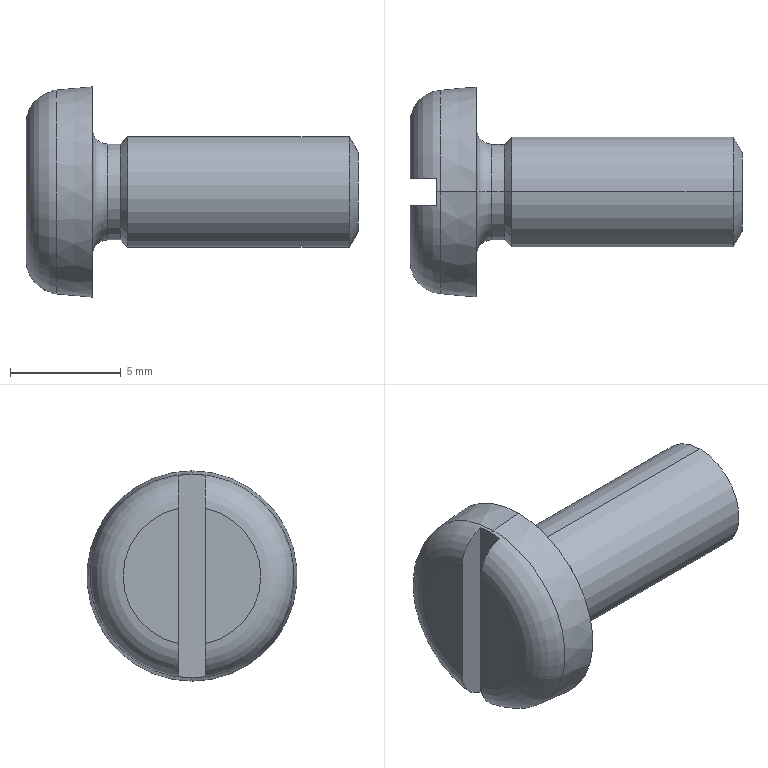Part | SolidWorks | features Cut 1, LPattern 1, RevCut 1, Revolution 1 | 1 solid | 21 faces | box 15 x 9.5 x 9.5 mm | volume 406.666 mm3 | plane 7 | cone 6 | cylinder 4 | torus 4 | commonest cylinder face diameters 4.33 x2 5 x2
STEP:
#1=CARTESIAN_POINT('',(15.,0.,-1.807));
#2=VERTEX_POINT('',#1);
#3=CARTESIAN_POINT('',(15.,0.,1.807));
#4=VERTEX_POINT('',#3);
#5=CARTESIAN_POINT('',(15.,0.,0.));
#6=DIRECTION('',(1.,0.,0.));
#7=DIRECTION('',(0.,0.,-1.));
#8=AXIS2_PLACEMENT_3D('',#5,#6,#7);
#9=CIRCLE('',#8,1.807);
#10=EDGE_CURVE('',#2,#4,#9,.T.);
#11=ORIENTED_EDGE('',*,*,#10,.F.);
#12=CARTESIAN_POINT('',(14.596,0.,-2.5));
#13=VERTEX_POINT('',#12);
#14=CARTESIAN_POINT('',(14.596,0.,-2.5));
#15=DIRECTION('',(-0.5041,0.,-0.8637));
#16=VECTOR('',#15,1000.);
#17=LINE('',#14,#16);
#18=EDGE_CURVE('',#2,#13,#17,.T.);
#19=ORIENTED_EDGE('',*,*,#18,.T.);
#20=CARTESIAN_POINT('',(14.596,0.,2.5));
#21=VERTEX_POINT('',#20);
#22=CARTESIAN_POINT('',(14.596,0.,0.));
#23=DIRECTION('',(1.,0.,0.));
#24=DIRECTION('',(0.,0.,-1.));
#25=AXIS2_PLACEMENT_3D('',#22,#23,#24);
#26=CIRCLE('',#25,2.5);
#27=EDGE_CURVE('',#13,#21,#26,.T.);
#28=ORIENTED_EDGE('',*,*,#27,.T.);
#29=CARTESIAN_POINT('',(14.596,0.,2.5));
#30=DIRECTION('',(-0.5041,0.,0.8637));
#31=VECTOR('',#30,1000.);
#32=LINE('',#29,#31);
#33=EDGE_CURVE('',#4,#21,#32,.T.);
#34=ORIENTED_EDGE('',*,*,#33,.F.);
#35=EDGE_LOOP('',(#11,#19,#28,#34));
#36=FACE_OUTER_BOUND('',#35,.T.);
#37=CARTESIAN_POINT('',(14.596,0.,0.));
#38=DIRECTION('',(-1.,0.,0.));
#39=DIRECTION('',(0.,0.,1.));
#40=AXIS2_PLACEMENT_3D('',#37,#38,#39);
#41=CONICAL_SURFACE('',#40,2.5,1.043);
#42=ADVANCED_FACE('',(#36),#41,.T.);
#43=ORIENTED_EDGE('',*,*,#27,.F.);
#44=CARTESIAN_POINT('',(4.6,0.,-2.5));
#45=VERTEX_POINT('',#44);
#46=CARTESIAN_POINT('',(-2.477,0.,-2.5));
#47=DIRECTION('',(-1.,0.,0.));
#48=VECTOR('',#47,1000.);
#49=LINE('',#46,#48);
#50=EDGE_CURVE('',#13,#45,#49,.T.);
#51=ORIENTED_EDGE('',*,*,#50,.T.);
#52=CARTESIAN_POINT('',(4.6,0.,2.5));
#53=VERTEX_POINT('',#52);
#54=CARTESIAN_POINT('',(4.6,0.,0.));
#55=DIRECTION('',(-1.,0.,0.));
#56=DIRECTION('',(0.,0.,1.));
#57=AXIS2_PLACEMENT_3D('',#54,#55,#56);
#58=CIRCLE('',#57,2.5);
#59=EDGE_CURVE('',#53,#45,#58,.T.);
#60=ORIENTED_EDGE('',*,*,#59,.F.);
#61=CARTESIAN_POINT('',(-2.477,0.,2.5));
#62=DIRECTION('',(-1.,0.,0.));
#63=VECTOR('',#62,1000.);
#64=LINE('',#61,#63);
#65=EDGE_CURVE('',#21,#53,#64,.T.);
#66=ORIENTED_EDGE('',*,*,#65,.F.);
#67=EDGE_LOOP('',(#43,#51,#60,#66));
#68=FACE_OUTER_BOUND('',#67,.T.);
#69=CARTESIAN_POINT('',(-2.477,0.,0.));
#70=DIRECTION('',(-1.,0.,0.));
#71=DIRECTION('',(0.,0.,1.));
#72=AXIS2_PLACEMENT_3D('',#69,#70,#71);
#73=CYLINDRICAL_SURFACE('',#72,2.5);
#74=ADVANCED_FACE('',(#68),#73,.T.);
#75=CARTESIAN_POINT('',(4.265,0.,2.165));
#76=VERTEX_POINT('',#75);
#77=CARTESIAN_POINT('',(4.265,0.,-2.165));
#78=VERTEX_POINT('',#77);
#79=CARTESIAN_POINT('',(4.265,0.,0.));
#80=DIRECTION('',(-1.,0.,0.));
#81=DIRECTION('',(0.,0.,1.));
#82=AXIS2_PLACEMENT_3D('',#79,#80,#81);
#83=CIRCLE('',#82,2.165);
#84=EDGE_CURVE('',#76,#78,#83,.T.);
#85=ORIENTED_EDGE('',*,*,#84,.F.);
#86=CARTESIAN_POINT('',(4.6,0.,2.5));
#87=DIRECTION('',(0.7071,0.,0.7071));
#88=VECTOR('',#87,1000.);
#89=LINE('',#86,#88);
#90=EDGE_CURVE('',#76,#53,#89,.T.);
#91=ORIENTED_EDGE('',*,*,#90,.T.);
#92=ORIENTED_EDGE('',*,*,#59,.T.);
#93=CARTESIAN_POINT('',(4.6,0.,-2.5));
#94=DIRECTION('',(0.7071,0.,-0.7071));
#95=VECTOR('',#94,1000.);
#96=LINE('',#93,#95);
#97=EDGE_CURVE('',#78,#45,#96,.T.);
#98=ORIENTED_EDGE('',*,*,#97,.F.);
#99=EDGE_LOOP('',(#85,#91,#92,#98));
#100=FACE_OUTER_BOUND('',#99,.T.);
#101=CARTESIAN_POINT('',(4.6,0.,0.));
#102=DIRECTION('',(1.,0.,0.));
#103=DIRECTION('',(0.,0.,-1.));
#104=AXIS2_PLACEMENT_3D('',#101,#102,#103);
#105=CONICAL_SURFACE('',#104,2.5,0.7854);
#106=ADVANCED_FACE('',(#100),#105,.T.);
#107=ORIENTED_EDGE('',*,*,#84,.T.);
#108=CARTESIAN_POINT('',(3.685,0.,-2.165));
#109=VERTEX_POINT('',#108);
#110=CARTESIAN_POINT('',(-2.477,0.,-2.165));
#111=DIRECTION('',(-1.,0.,0.));
#112=VECTOR('',#111,1000.);
#113=LINE('',#110,#112);
#114=EDGE_CURVE('',#78,#109,#113,.T.);
#115=ORIENTED_EDGE('',*,*,#114,.T.);
#116=CARTESIAN_POINT('',(3.685,0.,2.165));
#117=VERTEX_POINT('',#116);
#118=CARTESIAN_POINT('',(3.685,0.,0.));
#119=DIRECTION('',(-1.,0.,0.));
#120=DIRECTION('',(0.,0.,1.));
#121=AXIS2_PLACEMENT_3D('',#118,#119,#120);
#122=CIRCLE('',#121,2.165);
#123=EDGE_CURVE('',#117,#109,#122,.T.);
#124=ORIENTED_EDGE('',*,*,#123,.F.);
#125=CARTESIAN_POINT('',(-2.477,0.,2.165));
#126=DIRECTION('',(-1.,0.,0.));
#127=VECTOR('',#126,1000.);
#128=LINE('',#125,#127);
#129=EDGE_CURVE('',#76,#117,#128,.T.);
#130=ORIENTED_EDGE('',*,*,#129,.F.);
#131=EDGE_LOOP('',(#107,#115,#124,#130));
#132=FACE_OUTER_BOUND('',#131,.T.);
#133=CARTESIAN_POINT('',(-2.477,0.,0.));
#134=DIRECTION('',(-1.,0.,0.));
#135=DIRECTION('',(0.,0.,1.));
#136=AXIS2_PLACEMENT_3D('',#133,#134,#135);
#137=CYLINDRICAL_SURFACE('',#136,2.165);
#138=ADVANCED_FACE('',(#132),#137,.T.);
#139=CARTESIAN_POINT('',(3.,0.,-2.85));
#140=VERTEX_POINT('',#139);
#141=CARTESIAN_POINT('',(3.,0.,2.85));
#142=VERTEX_POINT('',#141);
#143=CARTESIAN_POINT('',(3.,0.,0.));
#144=DIRECTION('',(-1.,0.,0.));
#145=DIRECTION('',(0.,0.,1.));
#146=AXIS2_PLACEMENT_3D('',#143,#144,#145);
#147=CIRCLE('',#146,2.85);
#148=EDGE_CURVE('',#140,#142,#147,.T.);
#149=ORIENTED_EDGE('',*,*,#148,.F.);
#150=CARTESIAN_POINT('',(3.685,0.,-2.85));
#151=DIRECTION('',(0.,1.,0.));
#152=DIRECTION('',(0.,0.,1.));
#153=AXIS2_PLACEMENT_3D('',#150,#151,#152);
#154=CIRCLE('',#153,0.685);
#155=EDGE_CURVE('',#140,#109,#154,.T.);
#156=ORIENTED_EDGE('',*,*,#155,.T.);
#157=CARTESIAN_POINT('',(3.685,0.,0.));
#158=DIRECTION('',(-1.,0.,0.));
#159=DIRECTION('',(0.,0.,1.));
#160=AXIS2_PLACEMENT_3D('',#157,#158,#159);
#161=CIRCLE('',#160,2.165);
#162=EDGE_CURVE('',#109,#117,#161,.T.);
#163=ORIENTED_EDGE('',*,*,#162,.T.);
#164=CARTESIAN_POINT('',(3.685,0.,2.85));
#165=DIRECTION('',(0.,-1.,0.));
#166=DIRECTION('',(1.,0.,0.));
#167=AXIS2_PLACEMENT_3D('',#164,#165,#166);
#168=CIRCLE('',#167,0.685);
#169=EDGE_CURVE('',#142,#117,#168,.T.);
#170=ORIENTED_EDGE('',*,*,#169,.F.);
#171=EDGE_LOOP('',(#149,#156,#163,#170));
#172=FACE_OUTER_BOUND('',#171,.T.);
#173=CARTESIAN_POINT('',(3.685,0.,0.));
#174=DIRECTION('',(-1.,0.,0.));
#175=DIRECTION('',(0.,0.,1.));
#176=AXIS2_PLACEMENT_3D('',#173,#174,#175);
#177=TOROIDAL_SURFACE('',#176,2.85,0.685);
#178=ADVANCED_FACE('',(#172),#177,.F.);
#179=CARTESIAN_POINT('',(1.369,0.,4.607));
#180=VERTEX_POINT('',#179);
#181=CARTESIAN_POINT('',(1.369,0.,-4.607));
#182=VERTEX_POINT('',#181);
#183=CARTESIAN_POINT('',(1.369,0.,0.));
#184=DIRECTION('',(-1.,0.,0.));
#185=DIRECTION('',(0.,0.,1.));
#186=AXIS2_PLACEMENT_3D('',#183,#184,#185);
#187=CIRCLE('',#186,4.607);
#188=EDGE_CURVE('',#180,#182,#187,.T.);
#189=ORIENTED_EDGE('',*,*,#188,.F.);
#190=CARTESIAN_POINT('',(3.,0.,4.75));
#191=VERTEX_POINT('',#190);
#192=CARTESIAN_POINT('',(3.,0.,4.75));
#193=DIRECTION('',(0.9962,0.,0.08716));
#194=VECTOR('',#193,1000.);
#195=LINE('',#192,#194);
#196=EDGE_CURVE('',#180,#191,#195,.T.);
#197=ORIENTED_EDGE('',*,*,#196,.T.);
#198=CARTESIAN_POINT('',(3.,0.,-4.75));
#199=VERTEX_POINT('',#198);
#200=CARTESIAN_POINT('',(3.,0.,0.));
#201=DIRECTION('',(-1.,0.,0.));
#202=DIRECTION('',(0.,0.,1.));
#203=AXIS2_PLACEMENT_3D('',#200,#201,#202);
#204=CIRCLE('',#203,4.75);
#205=EDGE_CURVE('',#191,#199,#204,.T.);
#206=ORIENTED_EDGE('',*,*,#205,.T.);
#207=CARTESIAN_POINT('',(3.,0.,-4.75));
#208=DIRECTION('',(0.9962,0.,-0.08716));
#209=VECTOR('',#208,1000.);
#210=LINE('',#207,#209);
#211=EDGE_CURVE('',#182,#199,#210,.T.);
#212=ORIENTED_EDGE('',*,*,#211,.F.);
#213=EDGE_LOOP('',(#189,#197,#206,#212));
#214=FACE_OUTER_BOUND('',#213,.T.);
#215=CARTESIAN_POINT('',(3.,0.,0.));
#216=DIRECTION('',(1.,0.,0.));
#217=DIRECTION('',(0.,0.,-1.));
#218=AXIS2_PLACEMENT_3D('',#215,#216,#217);
#219=CONICAL_SURFACE('',#218,4.75,0.08727);
#220=ADVANCED_FACE('',(#214),#219,.T.);
#221=ORIENTED_EDGE('',*,*,#188,.T.);
#222=CARTESIAN_POINT('',(1.2,0.,-4.583));
#223=VERTEX_POINT('',#222);
#224=CARTESIAN_POINT('',(1.5,0.,-3.113));
#225=DIRECTION('',(0.,1.,0.));
#226=DIRECTION('',(0.,0.,1.));
#227=AXIS2_PLACEMENT_3D('',#224,#225,#226);
#228=CIRCLE('',#227,1.5);
#229=EDGE_CURVE('',#182,#223,#228,.T.);
#230=ORIENTED_EDGE('',*,*,#229,.T.);
#231=CARTESIAN_POINT('',(1.2,0.6,-4.543));
#232=VERTEX_POINT('',#231);
#233=CARTESIAN_POINT('',(1.2,0.,0.));
#234=DIRECTION('',(1.,0.,0.));
#235=DIRECTION('',(0.,1.,0.));
#236=AXIS2_PLACEMENT_3D('',#233,#234,#235);
#237=CIRCLE('',#236,4.583);
#238=EDGE_CURVE('',#223,#232,#237,.T.);
#239=ORIENTED_EDGE('',*,*,#238,.T.);
#240=CARTESIAN_POINT('',(0.,0.6,-3.055));
#241=VERTEX_POINT('',#240);
#242=CARTESIAN_POINT('',(1.2,0.6,-4.543));
#243=CARTESIAN_POINT('',(1.03,0.6,-4.508));
#244=CARTESIAN_POINT('',(0.8696,0.6,-4.445));
#245=CARTESIAN_POINT('',(0.5733,0.6,-4.263));
#246=CARTESIAN_POINT('',(0.4414,0.6,-4.146));
#247=CARTESIAN_POINT('',(0.2269,0.6,-3.878));
#248=CARTESIAN_POINT('',(0.1419,0.6,-3.724));
#249=CARTESIAN_POINT('',(0.0291,0.6,-3.4));
#250=CARTESIAN_POINT('',(0.,0.6,-3.226));
#251=CARTESIAN_POINT('',(0.,0.6,-3.055));
#252=B_SPLINE_CURVE_WITH_KNOTS('',3,(#242,#243,#244,#245,#246,#247,#248,#249,#250,#251),.UNSPECIFIED.,.F.,.F.,(4,2,2,2,4),(0.008666,0.00918,0.009694,0.01021,0.01072),.UNSPECIFIED.);
#253=EDGE_CURVE('',#232,#241,#252,.T.);
#254=ORIENTED_EDGE('',*,*,#253,.T.);
#255=CARTESIAN_POINT('',(0.,0.6,3.055));
#256=VERTEX_POINT('',#255);
#257=CARTESIAN_POINT('',(0.,0.,0.));
#258=DIRECTION('',(-1.,0.,0.));
#259=DIRECTION('',(0.,0.,1.));
#260=AXIS2_PLACEMENT_3D('',#257,#258,#259);
#261=CIRCLE('',#260,3.113);
#262=EDGE_CURVE('',#256,#241,#261,.T.);
#263=ORIENTED_EDGE('',*,*,#262,.F.);
#264=CARTESIAN_POINT('',(1.2,0.6,4.543));
#265=VERTEX_POINT('',#264);
#266=CARTESIAN_POINT('',(0.,0.6,3.055));
#267=CARTESIAN_POINT('',(0.,0.6,3.399));
#268=CARTESIAN_POINT('',(0.1194,0.6,3.744));
#269=CARTESIAN_POINT('',(0.4426,0.6,4.147));
#270=CARTESIAN_POINT('',(0.5742,0.6,4.264));
#271=CARTESIAN_POINT('',(0.868,0.6,4.444));
#272=CARTESIAN_POINT('',(1.031,0.6,4.509));
#273=CARTESIAN_POINT('',(1.2,0.6,4.543));
#274=B_SPLINE_CURVE_WITH_KNOTS('',3,(#266,#267,#268,#269,#270,#271,#272,#273),.UNSPECIFIED.,.F.,.F.,(4,2,2,4),(0.00147,0.0025,0.003015,0.00353),.UNSPECIFIED.);
#275=EDGE_CURVE('',#256,#265,#274,.T.);
#276=ORIENTED_EDGE('',*,*,#275,.T.);
#277=CARTESIAN_POINT('',(1.2,0.,4.583));
#278=VERTEX_POINT('',#277);
#279=CARTESIAN_POINT('',(1.2,0.,0.));
#280=DIRECTION('',(1.,0.,0.));
#281=DIRECTION('',(0.,1.,0.));
#282=AXIS2_PLACEMENT_3D('',#279,#280,#281);
#283=CIRCLE('',#282,4.583);
#284=EDGE_CURVE('',#265,#278,#283,.T.);
#285=ORIENTED_EDGE('',*,*,#284,.T.);
#286=CARTESIAN_POINT('',(1.5,0.,3.113));
#287=DIRECTION('',(0.,-1.,0.));
#288=DIRECTION('',(1.,0.,0.));
#289=AXIS2_PLACEMENT_3D('',#286,#287,#288);
#290=CIRCLE('',#289,1.5);
#291=EDGE_CURVE('',#180,#278,#290,.T.);
#292=ORIENTED_EDGE('',*,*,#291,.F.);
#293=EDGE_LOOP('',(#221,#230,#239,#254,#263,#276,#285,#292));
#294=FACE_OUTER_BOUND('',#293,.T.);
#295=CARTESIAN_POINT('',(1.5,0.,0.));
#296=DIRECTION('',(-1.,0.,0.));
#297=DIRECTION('',(0.,0.,1.));
#298=AXIS2_PLACEMENT_3D('',#295,#296,#297);
#299=TOROIDAL_SURFACE('',#298,3.113,1.5);
#300=ADVANCED_FACE('',(#294),#299,.T.);
#301=ORIENTED_EDGE('',*,*,#262,.T.);
#302=CARTESIAN_POINT('',(0.,0.6,-50.));
#303=DIRECTION('',(0.,0.,1.));
#304=VECTOR('',#303,1000.);
#305=LINE('',#302,#304);
#306=EDGE_CURVE('',#241,#256,#305,.T.);
#307=ORIENTED_EDGE('',*,*,#306,.T.);
#308=EDGE_LOOP('',(#301,#307));
#309=FACE_OUTER_BOUND('',#308,.T.);
#310=CARTESIAN_POINT('',(0.,3.113,0.));
#311=DIRECTION('',(1.,0.,0.));
#312=DIRECTION('',(0.,0.,-1.));
#313=AXIS2_PLACEMENT_3D('',#310,#311,#312);
#314=PLANE('',#313);
#315=ADVANCED_FACE('',(#309),#314,.F.);
#316=CARTESIAN_POINT('',(0.,-0.6,-3.055));
#317=VERTEX_POINT('',#316);
#318=CARTESIAN_POINT('',(0.,-0.6,3.055));
#319=VERTEX_POINT('',#318);
#320=CARTESIAN_POINT('',(0.,0.,0.));
#321=DIRECTION('',(-1.,0.,0.));
#322=DIRECTION('',(0.,0.,1.));
#323=AXIS2_PLACEMENT_3D('',#320,#321,#322);
#324=CIRCLE('',#323,3.113);
#325=EDGE_CURVE('',#317,#319,#324,.T.);
#326=ORIENTED_EDGE('',*,*,#325,.T.);
#327=CARTESIAN_POINT('',(0.,-0.6,-50.));
#328=DIRECTION('',(0.,0.,1.));
#329=VECTOR('',#328,1000.);
#330=LINE('',#327,#329);
#331=EDGE_CURVE('',#317,#319,#330,.T.);
#332=ORIENTED_EDGE('',*,*,#331,.F.);
#333=EDGE_LOOP('',(#326,#332));
#334=FACE_OUTER_BOUND('',#333,.T.);
#335=CARTESIAN_POINT('',(0.,3.113,0.));
#336=DIRECTION('',(1.,0.,0.));
#337=DIRECTION('',(0.,0.,-1.));
#338=AXIS2_PLACEMENT_3D('',#335,#336,#337);
#339=PLANE('',#338);
#340=ADVANCED_FACE('',(#334),#339,.F.);
#341=ORIENTED_EDGE('',*,*,#229,.F.);
#342=CARTESIAN_POINT('',(1.369,0.,0.));
#343=DIRECTION('',(-1.,0.,0.));
#344=DIRECTION('',(0.,0.,1.));
#345=AXIS2_PLACEMENT_3D('',#342,#343,#344);
#346=CIRCLE('',#345,4.607);
#347=EDGE_CURVE('',#182,#180,#346,.T.);
#348=ORIENTED_EDGE('',*,*,#347,.T.);
#349=ORIENTED_EDGE('',*,*,#291,.T.);
#350=CARTESIAN_POINT('',(1.2,-0.6,4.543));
#351=VERTEX_POINT('',#350);
#352=CARTESIAN_POINT('',(1.2,0.,0.));
#353=DIRECTION('',(1.,0.,0.));
#354=DIRECTION('',(0.,1.,0.));
#355=AXIS2_PLACEMENT_3D('',#352,#353,#354);
#356=CIRCLE('',#355,4.583);
#357=EDGE_CURVE('',#278,#351,#356,.T.);
#358=ORIENTED_EDGE('',*,*,#357,.T.);
#359=CARTESIAN_POINT('',(1.2,-0.6,4.543));
#360=CARTESIAN_POINT('',(1.031,-0.6,4.508));
#361=CARTESIAN_POINT('',(0.8686,-0.6,4.444));
#362=CARTESIAN_POINT('',(0.5738,-0.6,4.263));
#363=CARTESIAN_POINT('',(0.4433,-0.6,4.148));
#364=CARTESIAN_POINT('',(0.2266,-0.6,3.878));
#365=CARTESIAN_POINT('',(0.1427,-0.6,3.726));
#366=CARTESIAN_POINT('',(0.02866,-0.6,3.399));
#367=CARTESIAN_POINT('',(0.,-0.6,3.228));
#368=CARTESIAN_POINT('',(0.,-0.6,3.055));
#369=B_SPLINE_CURVE_WITH_KNOTS('',3,(#359,#360,#361,#362,#363,#364,#365,#366,#367,#368),.UNSPECIFIED.,.F.,.F.,(4,2,2,2,4),(0.005966,0.006481,0.006996,0.007512,0.008027),.UNSPECIFIED.);
#370=EDGE_CURVE('',#351,#319,#369,.T.);
#371=ORIENTED_EDGE('',*,*,#370,.T.);
#372=ORIENTED_EDGE('',*,*,#325,.F.);
#373=CARTESIAN_POINT('',(1.2,-0.6,-4.543));
#374=VERTEX_POINT('',#373);
#375=CARTESIAN_POINT('',(0.,-0.6,-3.055));
#376=CARTESIAN_POINT('',(0.,-0.6,-3.399));
#377=CARTESIAN_POINT('',(0.1181,-0.6,-3.743));
#378=CARTESIAN_POINT('',(0.443,-0.6,-4.148));
#379=CARTESIAN_POINT('',(0.575,-0.6,-4.264));
#380=CARTESIAN_POINT('',(0.8678,-0.6,-4.444));
#381=CARTESIAN_POINT('',(1.032,-0.6,-4.509));
#382=CARTESIAN_POINT('',(1.2,-0.6,-4.543));
#383=B_SPLINE_CURVE_WITH_KNOTS('',3,(#375,#376,#377,#378,#379,#380,#381,#382),.UNSPECIFIED.,.F.,.F.,(4,2,2,4),(0.008257,0.009287,0.009802,0.01032),.UNSPECIFIED.);
#384=EDGE_CURVE('',#317,#374,#383,.T.);
#385=ORIENTED_EDGE('',*,*,#384,.T.);
#386=CARTESIAN_POINT('',(1.2,0.,0.));
#387=DIRECTION('',(1.,0.,0.));
#388=DIRECTION('',(0.,1.,0.));
#389=AXIS2_PLACEMENT_3D('',#386,#387,#388);
#390=CIRCLE('',#389,4.583);
#391=EDGE_CURVE('',#374,#223,#390,.T.);
#392=ORIENTED_EDGE('',*,*,#391,.T.);
#393=EDGE_LOOP('',(#341,#348,#349,#358,#371,#372,#385,#392));
#394=FACE_OUTER_BOUND('',#393,.T.);
#395=CARTESIAN_POINT('',(1.5,0.,0.));
#396=DIRECTION('',(-1.,0.,0.));
#397=DIRECTION('',(0.,0.,1.));
#398=AXIS2_PLACEMENT_3D('',#395,#396,#397);
#399=TOROIDAL_SURFACE('',#398,3.113,1.5);
#400=ADVANCED_FACE('',(#394),#399,.T.);
#401=ORIENTED_EDGE('',*,*,#196,.F.);
#402=ORIENTED_EDGE('',*,*,#347,.F.);
#403=ORIENTED_EDGE('',*,*,#211,.T.);
#404=CARTESIAN_POINT('',(3.,0.,0.));
#405=DIRECTION('',(-1.,0.,0.));
#406=DIRECTION('',(0.,0.,1.));
#407=AXIS2_PLACEMENT_3D('',#404,#405,#406);
#408=CIRCLE('',#407,4.75);
#409=EDGE_CURVE('',#199,#191,#408,.T.);
#410=ORIENTED_EDGE('',*,*,#409,.T.);
#411=EDGE_LOOP('',(#401,#402,#403,#410));
#412=FACE_OUTER_BOUND('',#411,.T.);
#413=CARTESIAN_POINT('',(3.,0.,0.));
#414=DIRECTION('',(1.,0.,0.));
#415=DIRECTION('',(0.,0.,-1.));
#416=AXIS2_PLACEMENT_3D('',#413,#414,#415);
#417=CONICAL_SURFACE('',#416,4.75,0.08727);
#418=ADVANCED_FACE('',(#412),#417,.T.);
#419=ORIENTED_EDGE('',*,*,#409,.F.);
#420=ORIENTED_EDGE('',*,*,#205,.F.);
#421=EDGE_LOOP('',(#419,#420));
#422=FACE_OUTER_BOUND('',#421,.T.);
#423=CARTESIAN_POINT('',(3.,0.,0.));
#424=DIRECTION('',(-1.,0.,0.));
#425=DIRECTION('',(0.,0.,1.));
#426=AXIS2_PLACEMENT_3D('',#423,#424,#425);
#427=CIRCLE('',#426,2.85);
#428=EDGE_CURVE('',#142,#140,#427,.T.);
#429=ORIENTED_EDGE('',*,*,#428,.T.);
#430=ORIENTED_EDGE('',*,*,#148,.T.);
#431=EDGE_LOOP('',(#429,#430));
#432=FACE_BOUND('',#431,.T.);
#433=CARTESIAN_POINT('',(3.,2.85,0.));
#434=DIRECTION('',(-1.,0.,0.));
#435=DIRECTION('',(0.,0.,1.));
#436=AXIS2_PLACEMENT_3D('',#433,#434,#435);
#437=PLANE('',#436);
#438=ADVANCED_FACE('',(#422,#432),#437,.F.);
#439=ORIENTED_EDGE('',*,*,#155,.F.);
#440=ORIENTED_EDGE('',*,*,#428,.F.);
#441=ORIENTED_EDGE('',*,*,#169,.T.);
#442=ORIENTED_EDGE('',*,*,#123,.T.);
#443=EDGE_LOOP('',(#439,#440,#441,#442));
#444=FACE_OUTER_BOUND('',#443,.T.);
#445=CARTESIAN_POINT('',(3.685,0.,0.));
#446=DIRECTION('',(-1.,0.,0.));
#447=DIRECTION('',(0.,0.,1.));
#448=AXIS2_PLACEMENT_3D('',#445,#446,#447);
#449=TOROIDAL_SURFACE('',#448,2.85,0.685);
#450=ADVANCED_FACE('',(#444),#449,.F.);
#451=ORIENTED_EDGE('',*,*,#114,.F.);
#452=CARTESIAN_POINT('',(4.265,0.,0.));
#453=DIRECTION('',(-1.,0.,0.));
#454=DIRECTION('',(0.,0.,1.));
#455=AXIS2_PLACEMENT_3D('',#452,#453,#454);
#456=CIRCLE('',#455,2.165);
#457=EDGE_CURVE('',#78,#76,#456,.T.);
#458=ORIENTED_EDGE('',*,*,#457,.T.);
#459=ORIENTED_EDGE('',*,*,#129,.T.);
#460=ORIENTED_EDGE('',*,*,#162,.F.);
#461=EDGE_LOOP('',(#451,#458,#459,#460));
#462=FACE_OUTER_BOUND('',#461,.T.);
#463=CARTESIAN_POINT('',(-2.477,0.,0.));
#464=DIRECTION('',(-1.,0.,0.));
#465=DIRECTION('',(0.,0.,1.));
#466=AXIS2_PLACEMENT_3D('',#463,#464,#465);
#467=CYLINDRICAL_SURFACE('',#466,2.165);
#468=ADVANCED_FACE('',(#462),#467,.T.);
#469=ORIENTED_EDGE('',*,*,#90,.F.);
#470=ORIENTED_EDGE('',*,*,#457,.F.);
#471=ORIENTED_EDGE('',*,*,#97,.T.);
#472=CARTESIAN_POINT('',(4.6,0.,0.));
#473=DIRECTION('',(-1.,0.,0.));
#474=DIRECTION('',(0.,0.,1.));
#475=AXIS2_PLACEMENT_3D('',#472,#473,#474);
#476=CIRCLE('',#475,2.5);
#477=EDGE_CURVE('',#45,#53,#476,.T.);
#478=ORIENTED_EDGE('',*,*,#477,.T.);
#479=EDGE_LOOP('',(#469,#470,#471,#478));
#480=FACE_OUTER_BOUND('',#479,.T.);
#481=CARTESIAN_POINT('',(4.6,0.,0.));
#482=DIRECTION('',(1.,0.,0.));
#483=DIRECTION('',(0.,0.,-1.));
#484=AXIS2_PLACEMENT_3D('',#481,#482,#483);
#485=CONICAL_SURFACE('',#484,2.5,0.7854);
#486=ADVANCED_FACE('',(#480),#485,.T.);
#487=ORIENTED_EDGE('',*,*,#50,.F.);
#488=CARTESIAN_POINT('',(14.596,0.,0.));
#489=DIRECTION('',(1.,0.,0.));
#490=DIRECTION('',(0.,0.,-1.));
#491=AXIS2_PLACEMENT_3D('',#488,#489,#490);
#492=CIRCLE('',#491,2.5);
#493=EDGE_CURVE('',#21,#13,#492,.T.);
#494=ORIENTED_EDGE('',*,*,#493,.F.);
#495=ORIENTED_EDGE('',*,*,#65,.T.);
#496=ORIENTED_EDGE('',*,*,#477,.F.);
#497=EDGE_LOOP('',(#487,#494,#495,#496));
#498=FACE_OUTER_BOUND('',#497,.T.);
#499=CARTESIAN_POINT('',(-2.477,0.,0.));
#500=DIRECTION('',(-1.,0.,0.));
#501=DIRECTION('',(0.,0.,1.));
#502=AXIS2_PLACEMENT_3D('',#499,#500,#501);
#503=CYLINDRICAL_SURFACE('',#502,2.5);
#504=ADVANCED_FACE('',(#498),#503,.T.);
#505=CARTESIAN_POINT('',(1.2,0.6,-50.));
#506=DIRECTION('',(0.,0.,1.));
#507=VECTOR('',#506,1000.);
#508=LINE('',#505,#507);
#509=EDGE_CURVE('',#232,#265,#508,.T.);
#510=ORIENTED_EDGE('',*,*,#509,.T.);
#511=ORIENTED_EDGE('',*,*,#275,.F.);
#512=ORIENTED_EDGE('',*,*,#306,.F.);
#513=ORIENTED_EDGE('',*,*,#253,.F.);
#514=EDGE_LOOP('',(#510,#511,#512,#513));
#515=FACE_OUTER_BOUND('',#514,.T.);
#516=CARTESIAN_POINT('',(0.,0.6,-50.));
#517=DIRECTION('',(0.,1.,0.));
#518=DIRECTION('',(-1.,0.,0.));
#519=AXIS2_PLACEMENT_3D('',#516,#517,#518);
#520=PLANE('',#519);
#521=ADVANCED_FACE('',(#515),#520,.F.);
#522=ORIENTED_EDGE('',*,*,#509,.F.);
#523=ORIENTED_EDGE('',*,*,#238,.F.);
#524=ORIENTED_EDGE('',*,*,#391,.F.);
#525=CARTESIAN_POINT('',(1.2,-0.6,-50.));
#526=DIRECTION('',(0.,0.,1.));
#527=VECTOR('',#526,1000.);
#528=LINE('',#525,#527);
#529=EDGE_CURVE('',#374,#351,#528,.T.);
#530=ORIENTED_EDGE('',*,*,#529,.T.);
#531=ORIENTED_EDGE('',*,*,#357,.F.);
#532=ORIENTED_EDGE('',*,*,#284,.F.);
#533=EDGE_LOOP('',(#522,#523,#524,#530,#531,#532));
#534=FACE_OUTER_BOUND('',#533,.T.);
#535=CARTESIAN_POINT('',(1.2,0.6,-50.));
#536=DIRECTION('',(1.,0.,0.));
#537=DIRECTION('',(0.,1.,0.));
#538=AXIS2_PLACEMENT_3D('',#535,#536,#537);
#539=PLANE('',#538);
#540=ADVANCED_FACE('',(#534),#539,.F.);
#541=ORIENTED_EDGE('',*,*,#331,.T.);
#542=ORIENTED_EDGE('',*,*,#370,.F.);
#543=ORIENTED_EDGE('',*,*,#529,.F.);
#544=ORIENTED_EDGE('',*,*,#384,.F.);
#545=EDGE_LOOP('',(#541,#542,#543,#544));
#546=FACE_OUTER_BOUND('',#545,.T.);
#547=CARTESIAN_POINT('',(0.,-0.6,-50.));
#548=DIRECTION('',(0.,-1.,0.));
#549=DIRECTION('',(1.,0.,0.));
#550=AXIS2_PLACEMENT_3D('',#547,#548,#549);
#551=PLANE('',#550);
#552=ADVANCED_FACE('',(#546),#551,.F.);
#553=ORIENTED_EDGE('',*,*,#18,.F.);
#554=CARTESIAN_POINT('',(15.,0.,0.));
#555=DIRECTION('',(1.,0.,0.));
#556=DIRECTION('',(0.,0.,-1.));
#557=AXIS2_PLACEMENT_3D('',#554,#555,#556);
#558=CIRCLE('',#557,1.807);
#559=EDGE_CURVE('',#4,#2,#558,.T.);
#560=ORIENTED_EDGE('',*,*,#559,.F.);
#561=ORIENTED_EDGE('',*,*,#33,.T.);
#562=ORIENTED_EDGE('',*,*,#493,.T.);
#563=EDGE_LOOP('',(#553,#560,#561,#562));
#564=FACE_OUTER_BOUND('',#563,.T.);
#565=CARTESIAN_POINT('',(14.596,0.,0.));
#566=DIRECTION('',(-1.,0.,0.));
#567=DIRECTION('',(0.,0.,1.));
#568=AXIS2_PLACEMENT_3D('',#565,#566,#567);
#569=CONICAL_SURFACE('',#568,2.5,1.043);
#570=ADVANCED_FACE('',(#564),#569,.T.);
#571=ORIENTED_EDGE('',*,*,#559,.T.);
#572=ORIENTED_EDGE('',*,*,#10,.T.);
#573=EDGE_LOOP('',(#571,#572));
#574=FACE_OUTER_BOUND('',#573,.T.);
#575=CARTESIAN_POINT('',(15.,0.,0.));
#576=DIRECTION('',(-1.,0.,0.));
#577=DIRECTION('',(0.,0.,1.));
#578=AXIS2_PLACEMENT_3D('',#575,#576,#577);
#579=PLANE('',#578);
#580=ADVANCED_FACE('',(#574),#579,.F.);
#581=CLOSED_SHELL('',(#42,#74,#106,#138,#178,#220,#300,#315,#340,#400,#418,#438,#450,#468,#486,#504,#521,#540,#552,#570,#580));
#582=MANIFOLD_SOLID_BREP('',#581);
#583=CARTESIAN_POINT('',(0.,0.,0.));
#584=DIRECTION('',(0.,0.,1.));
#585=DIRECTION('',(1.,0.,0.));
#586=AXIS2_PLACEMENT_3D('',#583,#584,#585);
#587=(LENGTH_UNIT()NAMED_UNIT(*)SI_UNIT(.MILLI.,.METRE.));
#588=UNCERTAINTY_MEASURE_WITH_UNIT(LENGTH_MEASURE(0.00001),#587,'','');
#589=(NAMED_UNIT(*)PLANE_ANGLE_UNIT()SI_UNIT($,.RADIAN.));
#590=(NAMED_UNIT(*)SI_UNIT($,.STERADIAN.)SOLID_ANGLE_UNIT());
#591=(GEOMETRIC_REPRESENTATION_CONTEXT(3)GLOBAL_UNCERTAINTY_ASSIGNED_CONTEXT((#588))GLOBAL_UNIT_ASSIGNED_CONTEXT((#587,#589,#590))REPRESENTATION_CONTEXT('',''));
#592=ADVANCED_BREP_SHAPE_REPRESENTATION('',(#582,#586),#591);